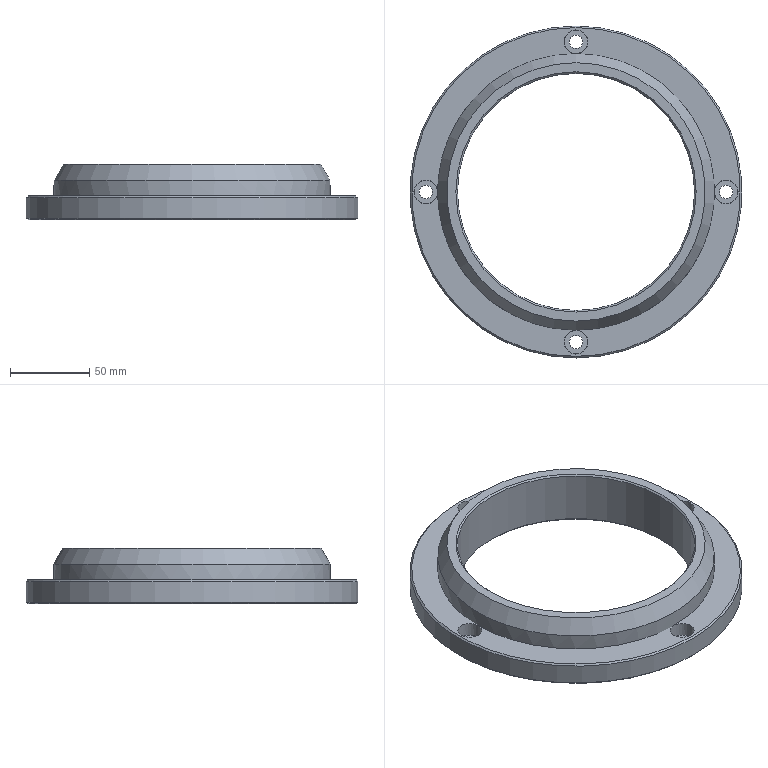Part | STEP file | solid 232 | 1 solid | 23 faces | box 210 x 210 x 35 mm | volume 357720 mm3 | cylinder 11 | plane 7 | cone 5 | commonest cylinder face diameters 8.5 x4 15 x4 150 x1 175 x1 210 x1